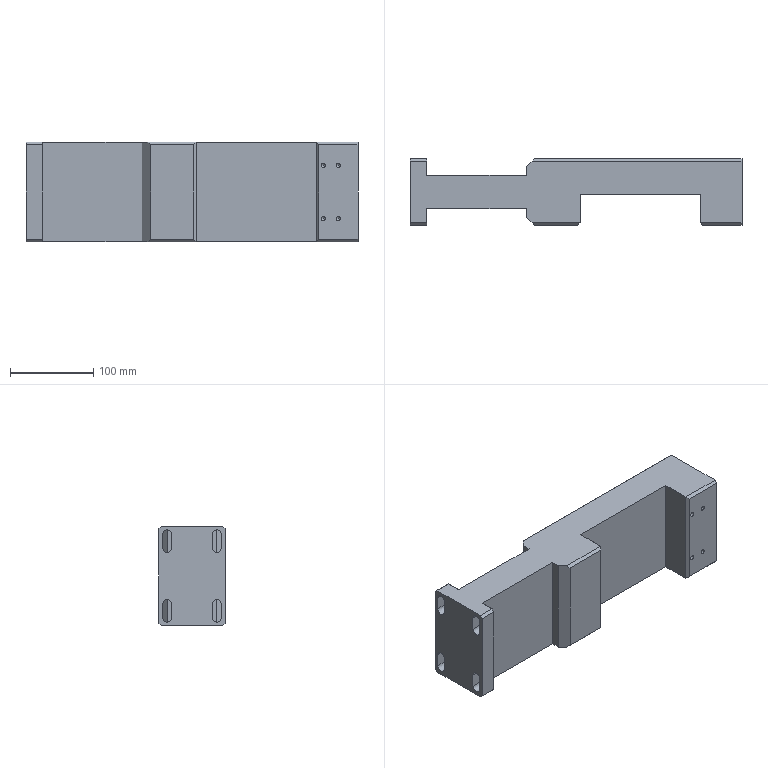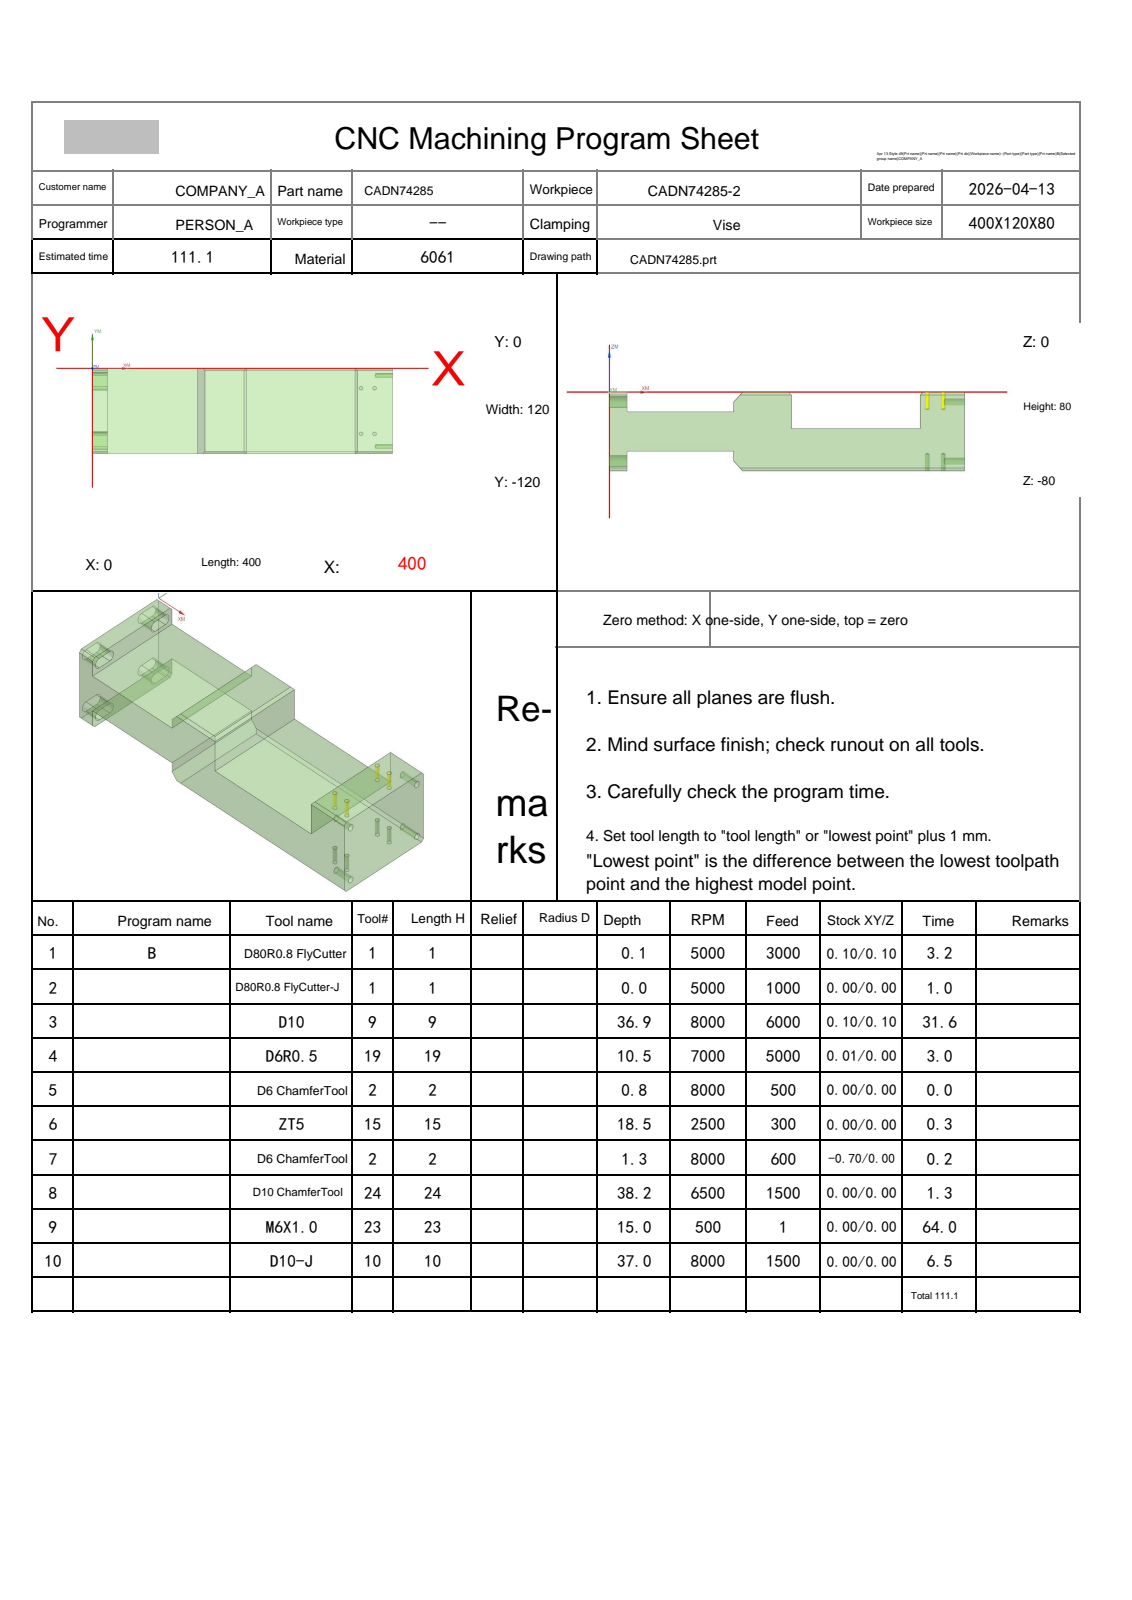NC program | NX | posted by the shop | part box 400 x 80 x 120 mm
Lines 9820 to 11018 of 11018:
N4 T19 M06
(D6R0.5  D=6. R=0.5 H=19 ce=0.01 di=0.00)
G00 G90 G54 X147.199 Y-123.373 M03 S7000
G43 H19 Z14.8
M08
Z.415
G01 Z-.085 F5000.
Y-118.246
Y-1.754
X147.116 Y-1.668 Z-.17
X147.113 Y-1.725
Y-118.275
X147.116 Y-118.332
X147.032 Y-118.417 Z-.255
X147.028 Y-118.275
Y-1.725
X147.032 Y-1.583
X146.947 Y-1.497 Z-.339
X146.943 Y-1.725
Y-118.275
X146.947 Y-118.503
X146.86 Y-118.588 Z-.424
X146.859 Y-117.278
Y-2.722
X146.86 Y-1.412
X146.776 Y-1.326 Z-.509
X146.774 Y-1.378
Y-118.622
X146.776 Y-118.674
X146.692 Y-118.759 Z-.594
X146.689 Y-118.622
Y-1.378
X146.692 Y-1.241
X146.607 Y-1.155 Z-.679
X146.604 Y-1.378
Y-118.622
X146.607 Y-118.844
X146.521 Y-118.93 Z-.764
X146.519 Y-117.617
Y-2.383
X146.521 Y-1.07
X146.437 Y-.985 Z-.849
X146.434 Y-1.031
Y-118.969
X146.437 Y-119.015
X146.353 Y-119.099 Z-.933
X146.35 Y-118.969
Y-1.031
X146.353 Y-.901
X146.268 Y-.816 Z-1.018
X146.265 Y-1.031
Y-118.969
X146.268 Y-119.184
X146.181 Y-119.269 Z-1.103
X146.18 Y-117.957
Y-2.043
X146.181 Y-.731
X146.097 Y-.646 Z-1.188
X146.095 Y-.684
Y-119.316
X146.097 Y-119.354
X146.013 Y-119.439 Z-1.273
X146.01 Y-119.316
Y-.684
X146.013 Y-.561
X145.929 Y-.477 Z-1.358
X145.925 Y-.684
Y-119.316
X145.929 Y-119.523
X145.842 Y-119.608 Z-1.442
X145.84 Y-118.296
Y-1.704
X145.842 Y-.392
X145.757 Y-.307 Z-1.527
X145.756 Y-.337
Y-119.663
X145.757 Y-119.693
X145.674 Y-119.777 Z-1.612
X145.671 Y-119.663
Y-.337
X145.674 Y-.222
X145.589 Y-.138 Z-1.697
X145.586 Y-.337
Y-119.663
X145.589 Y-119.862
X145.503 Y-119.946 Z-1.782
X145.501 Y-118.635
Y-1.365
X145.503 Y-.054
X145.417 Y.03 Z-1.867
X145.416 Y-1.28
Y-118.72
X145.417 Y-120.03
X145.334 Y-120.114 Z-1.952
X145.331 Y-120.009
Y.009
X145.334 Y.114
X145.25 Y.198 Z-2.036
X145.246 Y.009
Y-120.009
X145.25 Y-120.198
X145.164 Y-120.282 Z-2.121
X145.162 Y-118.975
Y-1.025
X145.164 Y.282
X145.077 Y.366 Z-2.206
Y-.94
Y-119.06
Y-120.366
X144.995 Y-120.45 Z-2.291
X144.992 Y-120.356
Y.356
X144.995 Y.45
X144.911 Y.534 Z-2.376
X144.907 Y.356
Y-120.356
X144.911 Y-120.534
X144.825 Y-120.618 Z-2.461
X144.822 Y-119.314
Y-.686
X144.825 Y.618
X144.737 Y.703 Z-2.546
Y-.601
Y-119.399
Y-120.703
X144.654 Y-120.787 Z-2.63
X144.652 Y-120.703
Y.703
X144.654 Y.787
X144.571 Y.87 Z-2.715
X144.568 Y.703
Y-120.703
X144.571 Y-120.87
X144.486 Y-120.954 Z-2.8
X144.483 Y-120.703
Y.703
X144.486 Y.954
X144.398 Y1.038 Z-2.885
Y-.261
Y-119.739
Y-121.038
X144.355 Y-121.05 Z-2.927
X144.314 Y-121.061 Z-2.97
X144.313 Y-119.823
Y-.177
X144.314 Y1.061
X144.271 Y1.062 Z-3.012
X144.229 Z-3.055
X144.228 Y-.092
Y-119.908
X144.229 Y-121.063
X144.186 Z-3.097
X144.144 Z-3.14
X144.143 Y-119.993
Y-.007
X144.144 Y1.063
X144.101 Y1.064 Z-3.182
X144.059 Z-3.224
X144.058 Y0.0
Y-120.
X144.059 Y-121.064
X144.016 Y-121.065 Z-3.267
X143.974 Z-3.309
Y-120.
Y0.0
Y1.065
X143.931 Y1.066 Z-3.352
X143.89 Z-3.394
X143.889 Y0.0
Y-120.
X143.89 Y-121.066
X143.846 Z-3.437
X143.805 Y-121.067 Z-3.479
X143.804 Y-120.
Y0.0
X143.805 Y1.067
X143.762 Z-3.521
X143.72 Y1.068 Z-3.564
X143.719 Y0.0
Y-120.
X143.72 Y-121.068
X143.677 Z-3.606
X143.635 Y-121.069 Z-3.649
X143.634 Y-120.
Y0.0
X143.635 Y1.069
X143.592 Z-3.691
X143.55 Z-3.734
X143.549 Y0.0
Y-120.
X143.55 Y-121.069
X143.507 Y-121.07 Z-3.776
X143.466 Z-3.818
X143.465 Y-120.
Y0.0
X143.466 Y1.07
X143.422 Y1.071 Z-3.861
X143.381 Z-3.903
X143.38 Y0.0
Y-120.
X143.381 Y-121.071
X143.337 Y-121.072 Z-3.946
X143.296 Z-3.988
X143.295 Y-120.
Y0.0
X143.296 Y1.072
X143.252 Y1.073 Z-4.031
X143.211 Z-4.073
X143.21 Y0.0
Y-120.
X143.211 Y-121.073
X143.168 Y-121.074 Z-4.115
X143.126 Z-4.158
X143.125 Y-120.
Y0.0
X143.126 Y1.074
X143.083 Z-4.2
X143.042 Y1.075 Z-4.243
X143.04 Y1.05
Y-121.05
X143.042 Y-121.075
X142.998 Z-4.285
X142.957 Y-121.076 Z-4.327
X142.955 Y-121.05
Y1.05
X142.957 Y1.076
X142.913 Z-4.37
X142.872 Y1.077 Z-4.412
X142.871 Y1.05
Y-121.05
X142.872 Y-121.077
X142.828 Z-4.455
X142.789 Z-4.497
X142.788 Y-121.05
Y1.05
X142.789 Y1.077
X142.743 Y1.078 Z-4.54
X142.702 Z-4.582
X142.701 Y1.05
Y-121.05
X142.702 Y-121.078
X142.658 Z-4.624
X142.617 Y-121.079 Z-4.667
X142.616 Y-121.05
Y1.05
X142.617 Y1.079
X142.574 Z-4.709
X142.533 Z-4.752
X142.531 Y1.05
Y-121.05
X142.533 Y-121.079
X142.489 Z-4.794
X142.448 Y-121.08 Z-4.837
X142.446 Y-121.05
Y1.05
X142.448 Y1.08
X142.404 Z-4.879
X142.363 Z-4.921
X142.361 Y1.05
Y-121.05
X142.363 Y-121.08
X142.319 Z-4.964
X142.278 Y-121.081 Z-5.006
X142.277 Y-121.05
Y1.05
X142.278 Y1.081
X142.234 Z-5.049
X142.193 Z-5.091
X142.192 Y1.05
Y-121.05
X142.193 Y-121.081
X142.149 Y-121.082 Z-5.134
X142.108 Z-5.176
X142.107 Y-121.05
Y1.05
X142.108 Y1.082
X142.064 Z-5.218
X142.024 Z-5.261
X142.022 Y1.05
Y-121.05
X142.024 Y-121.082
X141.98 Y-121.083 Z-5.303
X141.939 Z-5.346
X141.937 Y-121.05
Y1.05
X141.939 Y1.083
X141.895 Z-5.388
X141.854 Z-5.431
X141.852 Y1.05
Y-121.05
X141.854 Y-121.084
X141.81 Z-5.473
X141.769 Z-5.515
X141.767 Y-121.05
Y1.05
X141.769 Y1.084
X141.725 Z-5.558
X141.684 Y1.085 Z-5.6
X141.683 Y1.05
Y-121.05
X141.684 Y-121.085
X141.64 Z-5.643
X141.599 Z-5.685
X141.598 Y-121.05
Y1.05
X141.599 Y1.085
X141.555 Z-5.728
X141.515 Y1.086 Z-5.77
X141.513 Y1.05
Y-121.05
X141.515 Y-121.085
X141.47 Y-121.086 Z-5.812
X141.43 Z-5.855
X141.428 Y-121.05
Y1.05
X141.43 Y1.086
X141.386 Z-5.897
X141.345 Z-5.94
X141.343 Y1.05
Y-121.05
X141.345 Y-121.086
X141.301 Z-5.982
X141.26 Z-6.025
X141.258 Y-121.05
Y1.05
X141.26 Y1.086
X141.216 Z-6.067
X141.175 Y1.087 Z-6.109
X141.173 Y1.05
Y-121.05
X141.175 Y-121.086
X141.131 Z-6.152
X141.09 Z-6.194
X141.089 Y-121.05
Y1.05
X141.09 Y1.087
X141.046 Z-6.237
X141.006 Z-6.279
X141.004 Y1.05
Y-121.05
X141.006 Y-121.086
X140.961 Z-6.322
X140.921 Z-6.364
X140.919 Y-121.05
Y1.05
X140.921 Y1.087
X140.877 Z-6.406
X140.836 Z-6.449
X140.834 Y1.05
Y-121.05
X140.836 Y-121.086
X140.792 Z-6.491
X140.751 Z-6.534
X140.749 Y-121.05
Y1.05
X140.751 Y1.087
X140.707 Z-6.576
X140.666 Z-6.619
X140.664 Y1.05
Y-121.05
X140.666 Y-121.086
X140.622 Z-6.661
X140.581 Z-6.703
X140.58 Y-121.05
Y1.05
X140.581 Y1.087
X140.537 Z-6.746
X140.496 Z-6.788
X140.495 Y1.05
Y-121.05
X140.496 Y-121.086
X140.452 Z-6.831
X140.412 Z-6.873
X140.41 Y-121.05
Y1.05
X140.412 Y1.087
X140.367 Z-6.916
X140.327 Z-6.958
X140.325 Y1.05
Y-121.05
X140.327 Y-121.086
X140.283 Z-7.
X140.242 Z-7.043
X140.24 Y-121.05
Y1.05
X140.242 Y1.087
X140.198 Z-7.085
X140.156 Z-7.128
X140.155 Y0.0
Y-120.
X140.156 Y-121.086
X140.113 Z-7.17
X140.072 Z-7.212
X140.07 Y-121.05
Y1.05
X140.072 Y1.086
X140.028 Z-7.255
X139.987 Z-7.297
X139.986 Y1.05
Y-121.05
X139.987 Y-121.086
X139.943 Z-7.34
X139.902 Z-7.382
X139.901 Y-121.05
Y1.05
X139.902 Y1.086
X139.858 Y1.085 Z-7.425
X139.818 Z-7.467
X139.816 Y1.05
Y-121.05
X139.818 Y-121.085
X139.773 Z-7.509
X139.733 Z-7.552
X139.731 Y-121.05
Y1.05
X139.733 Y1.085
X139.689 Z-7.594
X139.648 Y1.084 Z-7.637
X139.646 Y1.05
Y-121.05
X139.648 Y-121.084
X139.604 Z-7.679
X139.563 Z-7.722
X139.561 Y-121.05
Y1.05
X139.563 Y1.084
X139.519 Z-7.764
X139.478 Y1.083 Z-7.806
X139.476 Y1.05
Y-121.05
X139.478 Y-121.083
X139.434 Z-7.849
X139.393 Z-7.891
X139.392 Y-121.05
Y1.05
X139.393 Y1.083
X139.349 Y1.082 Z-7.934
X139.308 Z-7.976
X139.307 Y1.05
Y-121.05
X139.308 Y-121.082
X139.264 Z-8.019
X139.223 Z-8.061
X139.222 Y-121.05
Y1.05
X139.223 Y1.082
X139.179 Y1.081 Z-8.103
X139.139 Z-8.146
X139.137 Y1.05
Y-121.05
X139.139 Y-121.081
X139.095 Z-8.188
X139.054 Z-8.231
X139.052 Y-121.05
Y1.05
X139.054 Y1.08
X139.01 Z-8.273
X138.969 Z-8.316
X138.967 Y1.05
Y-121.05
X138.969 Y-121.08
X138.925 Z-8.358
X138.884 Z-8.4
X138.882 Y-121.05
Y1.05
X138.884 Y1.079
X138.84 Z-8.443
X138.799 Z-8.485
X138.798 Y1.05
Y-121.05
X138.799 Y-121.079
X138.755 Z-8.528
X138.714 Y-121.078 Z-8.57
X138.713 Y-121.05
Y1.05
X138.714 Y1.078
X138.67 Z-8.613
X138.629 Z-8.655
X138.628 Y1.05
Y-121.05
X138.629 Y-121.078
X138.585 Y-121.077 Z-8.697
X138.544 Z-8.74
X138.543 Y-121.05
Y1.05
X138.544 Y1.077
X138.501 Y1.076 Z-8.782
X138.46 Z-8.825
X138.458 Y1.05
Y-121.05
X138.46 Y-121.076
X138.416 Z-8.867
X138.375 Y-121.075 Z-8.91
X138.373 Y-121.05
Y1.05
X138.375 Y1.075
X138.331 Z-8.952
X138.29 Y1.074 Z-8.994
X138.288 Y0.0
Y-120.
X138.29 Y-121.074
X138.246 Z-9.037
X138.205 Y-121.073 Z-9.079
X138.204 Y-120.
Y0.0
X138.205 Y1.073
X138.161 Z-9.122
X138.12 Y1.072 Z-9.164
X138.119 Y0.0
Y-120.
X138.12 Y-121.073
X138.076 Y-121.072 Z-9.207
X138.035 Z-9.249
X138.034 Y-120.
Y0.0
X138.035 Y1.072
X137.992 Y1.071 Z-9.291
X137.95 Z-9.334
X137.949 Y0.0
Y-120.
X137.95 Y-121.071
X137.907 Y-121.07 Z-9.376
X137.865 Z-9.419
X137.864 Y-120.
Y0.0
X137.865 Y1.07
X137.822 Z-9.461
X137.78 Y1.069 Z-9.504
X137.779 Y0.0
Y-120.
X137.78 Y-121.069
X137.737 Z-9.546
X137.696 Y-121.068 Z-9.588
X137.695 Y-120.
Y0.0
X137.696 Y1.068
X137.652 Z-9.631
X137.611 Y1.067 Z-9.673
X137.61 Y0.0
Y-120.
X137.611 Y-121.067
X137.567 Z-9.716
X137.526 Y-121.066 Z-9.758
X137.525 Y-120.
Y0.0
X137.526 Y1.066
X137.482 Z-9.801
X137.441 Z-9.843
X137.44 Y0.0
Y-120.
X137.441 Y-121.066
X137.398 Y-121.065 Z-9.885
X137.356 Z-9.928
X137.355 Y-120.
Y0.0
X137.356 Y1.065
X137.313 Y1.064 Z-9.97
X137.271 Z-10.013
X137.27 Y0.0
Y-120.
X137.271 Y-121.064
X137.228 Y-121.063 Z-10.055
X137.186 Z-10.097
X137.185 Y-119.949
Y-.051
X137.186 Y1.063
X137.143 Y1.062 Z-10.14
X137.101 Z-10.182
Y-121.062
X137.061 Y-121.06 Z-10.222
X137.022 Y-121.057 Z-10.262
Y1.057
X136.944 Y1.006 Z-10.341
Y-121.006
X136.866 Y-120.927 Z-10.421
Y.927
X136.787 Y.848 Z-10.5
Y-120.848
G00 Z14.8
G91 G28 Z0.0
M05
M09
G91 G28 Z0.0
M01
N5 T02 M06
(D6 ChamferTool  D=6. R=0. H=02 ce=0.00 di=0.00)
G00 G90 G54 X358. Y-28. M03 S8000
G43 H02 Z20.
M08
G98 G81 X358. Y-28. Z-.8 R1. F500.
X376.
Y-92.
X358.
G80
G00 Z20.
G91 G28 Z0.0
M05
M09
G91 G28 Z0.0
M01
N6 T15 M06
(ZT5 D=5. DR_a=118 H=15)
G00 G90 G54 X358. Y-28. M03 S2500
G43 H15 Z20.
M08
G98 G83 X358. Y-28. Z-18.502 R1. F300. Q3.
X376.
Y-92.
X358.
G80
G00 Z20.
G91 G28 Z0.0
M05
M09
G91 G28 Z0.0
M01
N7 T02 M06
(D6 ChamferTool  D=6. R=0. H=02 ce=-0.70 di=0.00)
G00 G90 G54 X357.13 Y-92.232 M03 S8000
G43 H02 Z20.
M08
Z-.8
G01 Z-1.3 F600.
X356.5 Y-92.4
G03 X358. Y-93.9 I1.5 J0.0
X359.9 Y-92. I0.0 J1.9
X358. Y-90.1 I-1.9 J0.0
X356.1 Y-92. I0.0 J-1.9
X358. Y-93.9 I1.9 J0.0
X359.5 Y-92.4 I0.0 J1.5
G01 X358.87 Y-92.232
Z-.8
G00 Z20.
X375.13
Z-.8
G01 Z-1.3
X374.5 Y-92.4
G03 X376. Y-93.9 I1.5 J0.0
X377.9 Y-92. I0.0 J1.9
X376. Y-90.1 I-1.9 J0.0
X374.1 Y-92. I0.0 J-1.9
X376. Y-93.9 I1.9 J0.0
X377.5 Y-92.4 I0.0 J1.5
G01 X376.87 Y-92.232
Z-.8
G00 Z20.
X375.13 Y-28.232
Z-.8
G01 Z-1.3
X374.5 Y-28.4
G03 X376. Y-29.9 I1.5 J0.0
X377.9 Y-28. I0.0 J1.9
X376. Y-26.1 I-1.9 J0.0
X374.1 Y-28. I0.0 J-1.9
X376. Y-29.9 I1.9 J0.0
X377.5 Y-28.4 I0.0 J1.5
G01 X376.87 Y-28.232
Z-.8
G00 Z20.
X357.13
Z-.8
G01 Z-1.3
X356.5 Y-28.4
G03 X358. Y-29.9 I1.5 J0.0
X359.9 Y-28. I0.0 J1.9
X358. Y-26.1 I-1.9 J0.0
X356.1 Y-28. I0.0 J-1.9
X358. Y-29.9 I1.9 J0.0
X359.5 Y-28.4 I0.0 J1.5
G01 X358.87 Y-28.232
Z-.8
G00 Z20.
G91 G28 Z0.0
M05
M09
G91 G28 Z0.0
M01
N8 T24 M06
(D10 ChamferTool  D=10. R=0. H=24 ce=0.00 di=0.00)
G00 G90 G54 X-.99 Y-117.792 M03 S6500
G43 H24 Z20.
M08
Z.13
G01 Z-1.2 F1500.
G03 X-.915 Y-117.452 I-1.907 J.601
G01 X-.905 Y-117.398
X-.928 Y-117.349
X-.966 Y-117.259
X-1. Y-117.
Y-3.
X-.966 Y-2.741
X-.928 Y-2.651
X-.905 Y-2.602
X-.915 Y-2.548
G03 X-.99 Y-2.208 I-1.983 J-.261
G01 Z.13
G00 Z10.
X20.99
Z.13
G01 Z-1.2
G03 X20.915 Y-2.548 I1.907 J-.601
G01 X20.905 Y-2.602
X20.928 Y-2.651
X20.966 Y-2.741
X21. Y-3.
Y-60.
Y-117.
X20.966 Y-117.259
X20.928 Y-117.349
X20.905 Y-117.398
X20.915 Y-117.452
G03 X20.99 Y-117.792 I1.983 J.261
G01 Z.13
G00 Z10.
X400.99 Y-2.208
Z.13
G01 Z-1.2
G03 X400.915 Y-2.548 I1.907 J-.601
G01 X400.905 Y-2.602
X400.928 Y-2.651
X400.966 Y-2.741
X401. Y-3.
Y-117.
X400.966 Y-117.259
X400.928 Y-117.349
X400.905 Y-117.398
X400.915 Y-117.452
G03 X400.99 Y-117.792 I1.983 J.261
G01 Z.13
G00 Z10.
X357.593 Y-29.315
Z.284
G01 Z-1.2
G03 X357.898 Y-29.484 I1.118 J1.658
G01 X357.946 Y-29.509
X358. Y-29.5
G03 X359.5 Y-28. I0.0 J1.5
X358. Y-26.5 I-1.5 J0.0
X356.5 Y-28. I0.0 J-1.5
X358. Y-29.5 I1.5 J0.0
G01 X358.054 Y-29.509
X358.102 Y-29.484
G03 X358.407 Y-29.315 I-.813 J1.827
G01 Z.284
G00 Z5.05
X375.593
Z.284
G01 Z-1.2
G03 X375.898 Y-29.484 I1.118 J1.658
G01 X375.946 Y-29.509
X376. Y-29.5
G03 X377.5 Y-28. I0.0 J1.5
X376. Y-26.5 I-1.5 J0.0
X374.5 Y-28. I0.0 J-1.5
X376. Y-29.5 I1.5 J0.0
G01 X376.054 Y-29.509
X376.102 Y-29.484
G03 X376.407 Y-29.315 I-.813 J1.827
G01 Z.284
G00 Z10.
X375.593 Y-93.315
Z.284
G01 Z-1.2
G03 X375.898 Y-93.484 I1.118 J1.658
G01 X375.946 Y-93.509
X376. Y-93.5
G03 X377.5 Y-92. I0.0 J1.5
X376. Y-90.5 I-1.5 J0.0
X374.5 Y-92. I0.0 J-1.5
X376. Y-93.5 I1.5 J0.0
G01 X376.054 Y-93.509
X376.102 Y-93.484
G03 X376.407 Y-93.315 I-.813 J1.827
G01 Z.284
G00 Z5.05
X357.593
Z.284
G01 Z-1.2
G03 X357.898 Y-93.484 I1.118 J1.658
G01 X357.946 Y-93.509
X358. Y-93.5
G03 X359.5 Y-92. I0.0 J1.5
X358. Y-90.5 I-1.5 J0.0
X356.5 Y-92. I0.0 J-1.5
X358. Y-93.5 I1.5 J0.0
G01 X358.054 Y-93.509
X358.102 Y-93.484
G03 X358.407 Y-93.315 I-.813 J1.827
G01 Z.284
G00 Z10.
X134.933 Y-121.068
Z-13.097
G01 Z-21.2
X134.848 Y-121.008
X134.818 Y-121.
X25.156
X25.136 Y-121.005
X25.079 Y-121.045
Z-4.635
G00 Z10.
X25.067 Y1.068
Z-4.641
G01 Z-21.2
X25.152 Y1.008
X25.182 Y1.
X134.844
X134.864 Y1.005
X134.921 Y1.045
Z-13.105
G00 Z10.
X210.066 Y1.068
Z-6.301
G01 Z-38.2
X210.152 Y1.008
X210.182 Y1.
X344.818
X344.848 Y1.008
X344.934 Y1.068
Z-6.301
G00 Z10.
Y-121.068
Z-6.301
G01 Z-38.2
X344.848 Y-121.008
X344.818 Y-121.
X210.182
X210.152 Y-121.008
X210.066 Y-121.068
Z-6.301
G00 Z20.
G00 G90 X405.7 Y-121.028 M03 S6500
Z20.
Z-2.2
G01 Z-3.7 F1500.
G03 X404.603 Y-120.7 I-1.097 J-1.672
G01 X349.3
Y.7
X404.603
G03 X405.7 Y1.028 I0.0 J2.
G01 Z-2.2
G00 Z20.
X140.397 Y2.7
Z-2.2
G01 Z-3.7
G03 X142.397 Y.7 I2. J0.0
G01 X205.7
Y-120.7
X142.397
G03 X140.397 Y-122.7 I0.0 J-2.
G01 Z-2.2
G00 Z20.
X-5.7 Y1.028
Z-2.2
G01 Z-3.7
G03 X-4.603 Y.7 I1.097 J1.672
G01 X25.71
G03 X27.71 Y2.7 I0.0 J2.
G01 Z-2.2
G00 Z20.
Y-122.7
Z-2.2
G01 Z-3.7
G03 X25.71 Y-120.7 I-2. J0.0
G01 X-4.603
G03 X-5.7 Y-121.028 I0.0 J-2.
G01 Z-2.2
G00 Z20.
G91 G28 Z0.0
M05
M09
G91 G28 Z0.0
M01
N9 T23 M06
(M6X1.0 D=5. DR_a=180 H=23)
G00 G90 G54 X358. Y-28. M03 S500
G43 H23 Z20.
M08
G95
G98 G84 X358. Y-28. Z-15. R1. F1. Q3.
X376.
Y-92.
X358.
G80
G94
G00 Z20.
G91 G28 Z0.0
M05
M09
G91 G28 Z0.0
M01
N10 T10 M06
(D10-J  D=10. R=0. H=10 ce=0.40 di=0.00)
G00 G90 G54 X23.402 Y-127. M03 S8000
G43 H10 Z14.8
M08
Z-18.5
G01 Z-20. F1000.
G03 X25.401 Y-125. I-.001 J2.
G01 Y4.1
G02 X26.301 Y5. I.9 J0.0
G01 X29.365
G02 X30.365 Y4. I0.0 J-1.
G01 Y-124.1
G03 X31.265 Y-125. I.9 J0.0
G01 X34.328
G03 X35.328 Y-124. I0.0 J1.
G01 Y4.1
G02 X36.228 Y5. I.9 J0.0
G01 X39.292
G02 X40.292 Y4. I0.0 J-1.
G01 Y-124.1
G03 X41.192 Y-125. I.9 J0.0
G01 X44.255
G03 X45.255 Y-124. I0.0 J1.
G01 Y4.1
G02 X46.155 Y5. I.9 J0.0
G01 X49.219
G02 X50.219 Y4. I0.0 J-1.
G01 Y-124.1
G03 X51.119 Y-125. I.9 J0.0
G01 X54.183
G03 X55.183 Y-124. I0.0 J1.
G01 Y4.1
G02 X56.083 Y5. I.9 J0.0
G01 X59.146
G02 X60.146 Y4. I0.0 J-1.
G01 Y-124.1
G03 X61.046 Y-125. I.9 J0.0
G01 X64.11
G03 X65.11 Y-124. I0.0 J1.
G01 Y4.
G02 X66.11 Y5. I1. J0.0
G01 X69.173
G02 X70.073 Y4.1 I0.0 J-.9
G01 Y-124.1
G03 X70.973 Y-125. I.9 J0.0
G01 X74.037
G03 X75.037 Y-124. I0.0 J1.
G01 Y4.
G02 X76.037 Y5. I1. J0.0
G01 X79.1
G02 X80. Y4.1 I0.0 J-.9
G01 Y-124.
G03 X81. Y-125. I1. J0.0
G01 X84.064
G03 X84.964 Y-124.1 I0.0 J.9
G01 Y4.1
G02 X85.864 Y5. I.9 J0.0
G01 X88.928
G02 X89.928 Y4. I0.0 J-1.
G01 Y-124.1
G03 X90.828 Y-125. I.9 J0.0
G01 X93.891
G03 X94.891 Y-124. I0.0 J1.
G01 Y4.1
G02 X95.791 Y5. I.9 J0.0
G01 X98.855
G02 X99.855 Y4. I0.0 J-1.
G01 Y-124.1
G03 X100.755 Y-125. I.9 J0.0
G01 X103.818
G03 X104.818 Y-124. I0.0 J1.
G01 Y4.1
G02 X105.718 Y5. I.9 J0.0
G01 X108.782
G02 X109.782 Y4. I0.0 J-1.
G01 Y-124.1
G03 X110.682 Y-125. I.9 J0.0
G01 X113.746
G03 X114.746 Y-124. I0.0 J1.
G01 Y4.1
G02 X115.646 Y5. I.9 J0.0
G01 X118.709
G02 X119.709 Y4. I0.0 J-1.
G01 Y-124.1
G03 X120.609 Y-125. I.9 J0.0
G01 X123.673
G03 X124.673 Y-124. I0.0 J1.
G01 Y4.1
G02 X125.573 Y5. I.9 J0.0
G01 X128.636
G02 X129.636 Y4. I0.0 J-1.
G01 Y-124.1
G03 X130.536 Y-125. I.9 J0.0
G01 X133.6
G03 X134.6 Y-124. I0.0 J1.
G01 Y5.
G03 X132.601 Y7. I-2. J0.0
G01 Z-18.5
G00 Z14.8
G00 G90 X208.402 Y-127. M03 S7000
Z14.8
Z-35.5
G01 Z-37. F1500.
G03 X210.401 Y-125. I-.001 J2.
G01 Y4.1
G02 X211.301 Y5. I.9 J0.0
G01 X214.371
G02 X215.371 Y4. I0.0 J-1.
G01 Y-124.1
G03 X216.271 Y-125. I.9 J0.0
G01 X219.342
G03 X220.342 Y-124. I0.0 J1.
G01 Y4.1
G02 X221.242 Y5. I.9 J0.0
G01 X224.312
G02 X225.312 Y4. I0.0 J-1.
G01 Y-124.1
G03 X226.212 Y-125. I.9 J0.0
G01 X229.282
G03 X230.282 Y-124. I0.0 J1.
G01 Y4.1
G02 X231.182 Y5. I.9 J0.0
G01 X234.253
G02 X235.253 Y4. I0.0 J-1.
G01 Y-124.1
G03 X236.153 Y-125. I.9 J0.0
G01 X239.223
G03 X240.223 Y-124. I0.0 J1.
G01 Y4.1
G02 X241.123 Y5. I.9 J0.0
G01 X244.193
G02 X245.193 Y4. I0.0 J-1.
G01 Y-124.1
G03 X246.093 Y-125. I.9 J0.0
G01 X249.164
G03 X250.164 Y-124. I0.0 J1.
G01 Y4.1
G02 X251.064 Y5. I.9 J0.0
G01 X254.134
G02 X255.134 Y4. I0.0 J-1.
G01 Y-124.1
G03 X256.034 Y-125. I.9 J0.0
G01 X259.104
G03 X260.104 Y-124. I0.0 J1.
G01 Y4.1
G02 X261.004 Y5. I.9 J0.0
G01 X264.075
G02 X265.075 Y4. I0.0 J-1.
G01 Y-124.1
G03 X265.975 Y-125. I.9 J0.0
G01 X269.045
G03 X270.045 Y-124. I0.0 J1.
G01 Y4.1
G02 X270.945 Y5. I.9 J0.0
G01 X274.015
G02 X275.015 Y4. I0.0 J-1.
G01 Y-124.1
G03 X275.915 Y-125. I.9 J0.0
G01 X278.986
G03 X279.986 Y-124. I0.0 J1.
G01 Y4.1
G02 X280.886 Y5. I.9 J0.0
G01 X283.956
G02 X284.956 Y4. I0.0 J-1.
G01 Y-124.1
G03 X285.856 Y-125. I.9 J0.0
G01 X288.926
G03 X289.926 Y-124. I0.0 J1.
G01 Y4.1
G02 X290.826 Y5. I.9 J0.0
G01 X293.897
G02 X294.897 Y4. I0.0 J-1.
G01 Y-124.1
G03 X295.797 Y-125. I.9 J0.0
G01 X298.867
G03 X299.867 Y-124. I0.0 J1.
G01 Y4.1
G02 X300.767 Y5. I.9 J0.0
G01 X303.837
G02 X304.837 Y4. I0.0 J-1.
G01 Y-124.1
G03 X305.737 Y-125. I.9 J0.0
G01 X308.808
G03 X309.808 Y-124. I0.0 J1.
G01 Y4.1
G02 X310.708 Y5. I.9 J0.0
G01 X313.778
G02 X314.778 Y4. I0.0 J-1.
G01 Y-124.1
G03 X315.678 Y-125. I.9 J0.0
G01 X318.748
G03 X319.748 Y-124. I0.0 J1.
G01 Y4.1
G02 X320.648 Y5. I.9 J0.0
G01 X323.719
G02 X324.719 Y4. I0.0 J-1.
G01 Y-124.1
G03 X325.619 Y-125. I.9 J0.0
G01 X328.689
G03 X329.689 Y-124. I0.0 J1.
G01 Y4.1
G02 X330.589 Y5. I.9 J0.0
G01 X333.659
G02 X334.659 Y4. I0.0 J-1.
G01 Y-124.1
G03 X335.559 Y-125. I.9 J0.0
G01 X338.63
G03 X339.63 Y-124. I0.0 J1.
G01 Y4.1
G02 X340.53 Y5. I.9 J0.0
G01 X343.6
G02 X344.6 Y4. I0.0 J-1.
G01 Y-125.
G02 X342.601 Y-127. I-2. J0.0
G01 Z-35.5
G00 Z14.8
G00 G90 X138.468 Y-127.191 M03 S8000
Z14.8
Z-19.
G01 Z-20. F1000.
G41 D10
X138.527 Y-127.
G03 X138.615 Y-126.414 I-1.912 J.586
X138.029 Y-125. I-2. J0.0
G01 X135. Y-121.971
Y1.971
X138.029 Y5.
G03 X138.615 Y6.414 I-1.414 J1.414
X138.527 Y7. I-2. J0.0
G01 G40 X138.468 Y7.191
Z-19.
G00 X21.532
G01 Z-20.
G41 D10
X21.473 Y7.
G03 X21.385 Y6.414 I1.912 J-.586
X21.971 Y5. I2. J0.0
G01 X25. Y1.971
Y-121.971
X21.971 Y-125.
G03 X21.385 Y-126.414 I1.414 J-1.414
X21.473 Y-127. I2. J0.0
G01 G40 X21.532 Y-127.191
Z-19.
G00 Z14.8
G00 G90 X206.532 Y7.191 M03 S8000
Z14.8
Z-17.5
G01 Z-18.5 F1000.
G41 D10
X206.473 Y7.
G03 X206.385 Y6.414 I1.912 J-.586
X206.971 Y5. I2. J0.0
G01 X210. Y1.971
Y-121.971
X206.971 Y-125.
G03 X206.385 Y-126.414 I1.414 J-1.414
X206.473 Y-127. I2. J0.0
G01 G40 X206.532 Y-127.191
Z-17.5
G00 X348.468
G01 Z-18.5
G41 D10
X348.527 Y-127.
G03 X348.615 Y-126.414 I-1.912 J.586
X348.029 Y-125. I-2. J0.0
G01 X345. Y-121.971
Y1.971
X348.029 Y5.
G03 X348.615 Y6.414 I-1.414 J1.414
X348.527 Y7. I-2. J0.0
G01 G40 X348.468 Y7.191
Z-17.5
G00 Z14.8
Y-127.191
Z-36.
G01 Z-37.
G41 D10
X348.527 Y-127.
G03 X348.615 Y-126.414 I-1.912 J.586
X348.029 Y-125. I-2. J0.0
G01 X345. Y-121.971
Y1.971
X348.029 Y5.
G03 X348.615 Y6.414 I-1.414 J1.414
X348.527 Y7. I-2. J0.0
G01 G40 X348.468 Y7.191
Z-36.
G00 X206.532
G01 Z-37.
G41 D10
X206.473 Y7.
G03 X206.385 Y6.414 I1.912 J-.586
X206.971 Y5. I2. J0.0
G01 X210. Y1.971
Y-121.971
X206.971 Y-125.
G03 X206.385 Y-126.414 I1.414 J-1.414
X206.473 Y-127. I2. J0.0
G01 G40 X206.532 Y-127.191
Z-36.
G00 Z14.8
M05
M09
G91 G28 Z0.0
G91 G28 Y0.0
M30
%